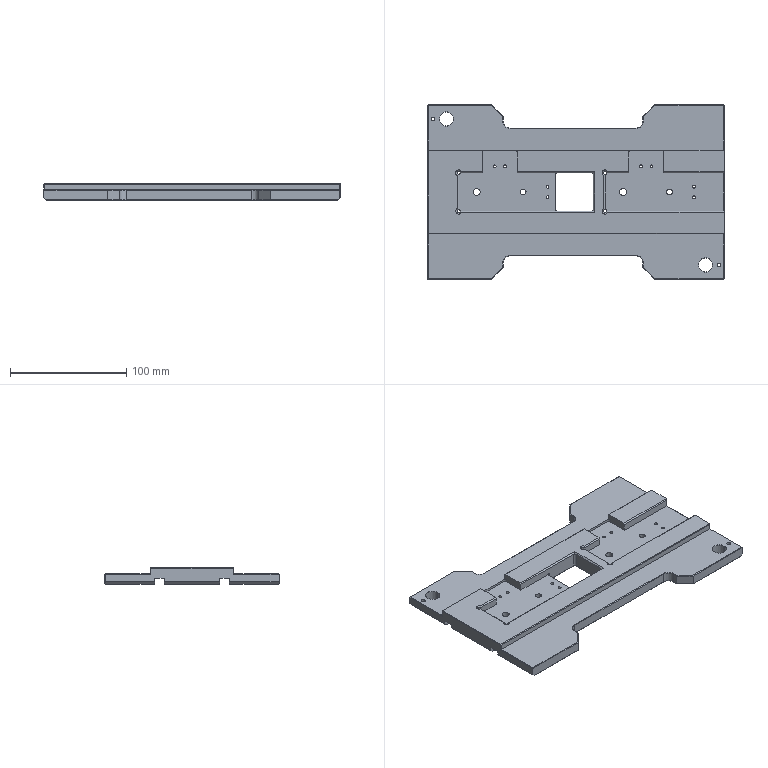Part | STEP file | base hole locating fixture plate | 1 solid | 217 faces | box 255 x 150 x 14 mm | volume 299894 mm3 | plane 131 | cylinder 60 | cone 26 | commonest cylinder face diameters 2.5 x16 3 x8 4 x8 6 x8 12 x8 3.3 x4